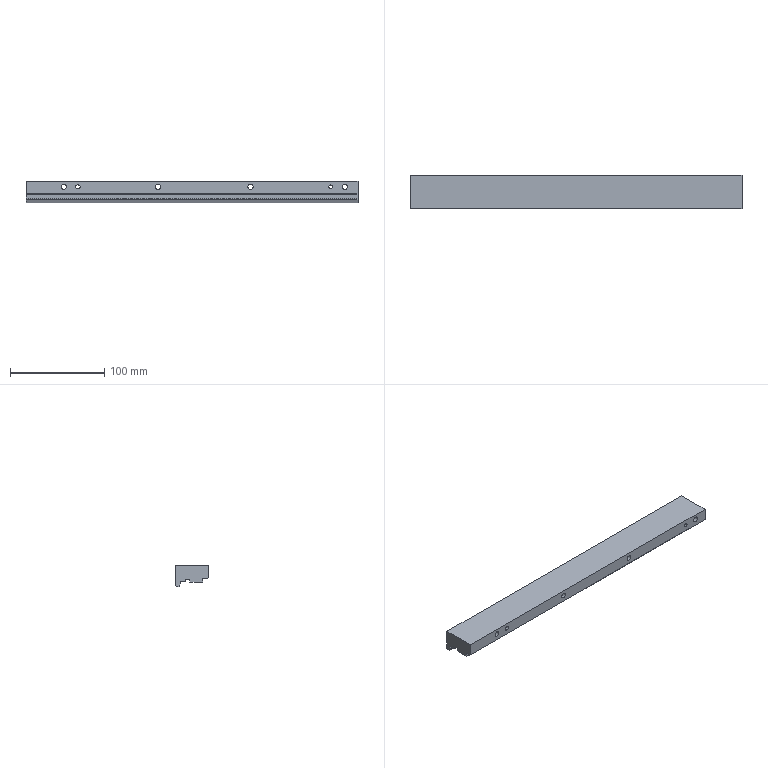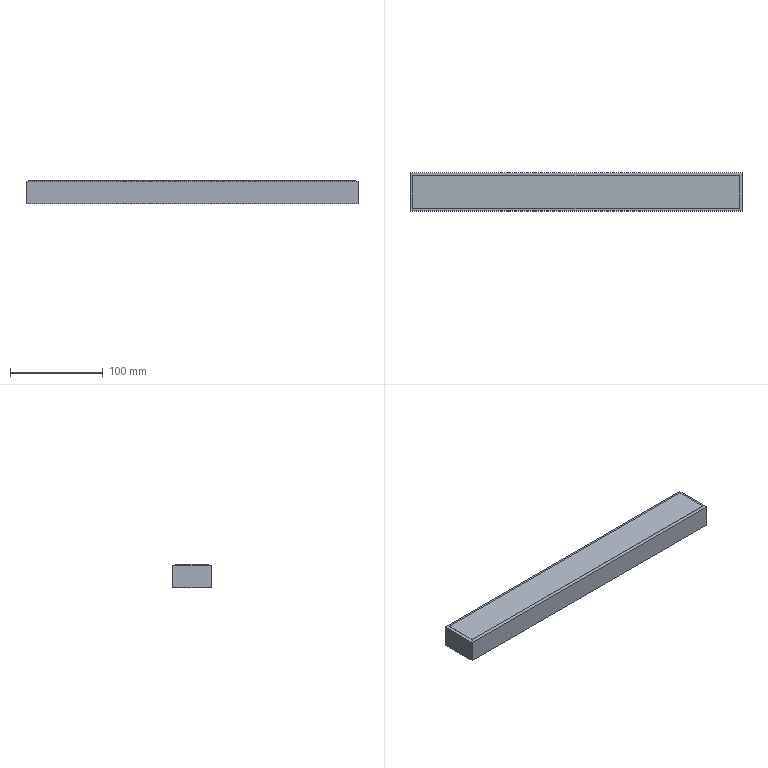CAM job | NX | 3-axis milling | part box 352 x 35 x 22.9 mm | stock box 358 x 41 x 24.9 mm
Tools:
number,name,description,diameter,corner_radius,flute_length,length,flutes
1,D50,Milling Tool-5 Parameters,50.0,0.0,50.0,75.0,2
3,D10,Milling Tool-5 Parameters,10.0,0.0,50.0,75.0,2
4,D10JING,Milling Tool-5 Parameters,10.0,0.0,50.0,75.0,2
2,D6A45,Milling Tool-5 Parameters,6.0,0.0,3.0,3.0,2
8,D6,Milling Tool-5 Parameters,6.0,0.0,50.0,75.0,2
10,D4,Milling Tool-5 Parameters,4.0,0.0,50.0,75.0,2
20,D6R0.5,Milling Tool-5 Parameters,6.0,0.5,50.0,75.0,2
Operations:
program,operation,operation_type,tool,method,geometry_group,spindle_rpm,surface_speed,feed_per_tooth,feed_cut,feed_plunge,cut_length_mm,path_length_mm,cut_time_min,machine_time_min
1-357-40-25毛胚,FLOOR_WALL,VolumeBased25DMillingOperation,D50,METHOD,A,6500.0,1286.0,0.0962,1250.0,100.0,420.0,474.0,0.336,0.3414
1-357-40-25毛胚,ZLEVEL_PROFILE,ZLevelMilling,D10,METHOD,A,7000.0,219.0,0.2143,3000.0,1000.0,18645.435,18725.335,6.247,6.255
1-357-40-25毛胚,ZLEVEL_PROFILE_COPY_COPY_1_COPY_COPY_COPY_1,ZLevelMilling,D10JING,METHOD,A,7000.0,219.0,0.0714,1000.0,100.0,1617.097,1723.116,1.617,1.628
1-357-40-25毛胚,ZLEVEL_PROFILE_COPY_1_COPY_COPY_COPY_COPY_2_COPY,ZLevelMilling,D6A45,METHOD,A,7000.0,131.0,0.0714,1000.0,1000.0,783.121,845.121,0.7831,0.7893
2-357-40-25毛胚,FLOOR_WALL_COPY,VolumeBased25DMillingOperation,D50,METHOD,B,6500.0,1286.0,0.0962,1250.0,100.0,828.0,1342,0.6624,0.7138
2-357-40-25毛胚,FLOOR_WALL_1,VolumeBased25DMillingOperation,D10,METHOD,B,7000.0,219.0,0.2143,3000.0,1000.0,2554.061,2625.361,0.8554,0.8625
2-357-40-25毛胚,FLOOR_WALL_1_COPY,VolumeBased25DMillingOperation,D10,METHOD,B,7000.0,219.0,0.2143,3000.0,1000.0,8723.15,8786.85,2.912,2.918
2-357-40-25毛胚,FLOOR_WALL_1_COPY_1_1,VolumeBased25DMillingOperation,D6,METHOD,B,7000.0,87.0,0.0714,1000.0,100.0,5076.709,6015.516,5.077,5.195
2-357-40-25毛胚,FLOOR_WALL_1_1,VolumeBased25DMillingOperation,D4,METHOD,B,7000.0,87.0,0.1429,2000.0,1000.0,5023.9,5097.6,2.534,2.541
2-357-40-25毛胚,FLOOR_WALL_1_COPY_1,VolumeBased25DMillingOperation,D4,METHOD,B,7000.0,87.0,0.0714,1000.0,100.0,1449.599,1525.999,1.45,1.457
2-357-40-25毛胚,ZLEVEL_PROFILE_COPY_COPY_1_COPY_COPY_COPY_1_COPY_COPY,ZLevelMilling,D6R0.5,METHOD,B,7000.0,131.0,0.2143,3000.0,1000.0,13770.416,13834.007,4.591,4.597
2-357-40-25毛胚,ZLEVEL_PROFILE_COPY_1_COPY_COPY_COPY_COPY_2_COPY_COPY_COPY_COPY,ZLevelMilling,D6A45,METHOD,B,7000.0,131.0,0.0714,1000.0,1000.0,372.653,435.653,0.3727,0.379
2-357-40-25毛胚,ZLEVEL_PROFILE_COPY_1_COPY_COPY_COPY_COPY_2_COPY_COPY,ZLevelMilling,D6A45,METHOD,B,7000.0,131.0,0.0714,1000.0,1000.0,1104.735,1606.68,1.105,1.155
2-357-40-25毛胚,ZLEVEL_PROFILE_COPY_1_COPY_COPY_COPY_COPY_2_COPY_COPY_COPY,ZLevelMilling,D6A45,METHOD,B,7000.0,131.0,0.0714,1000.0,1000.0,368.898,450.498,0.3689,0.3771